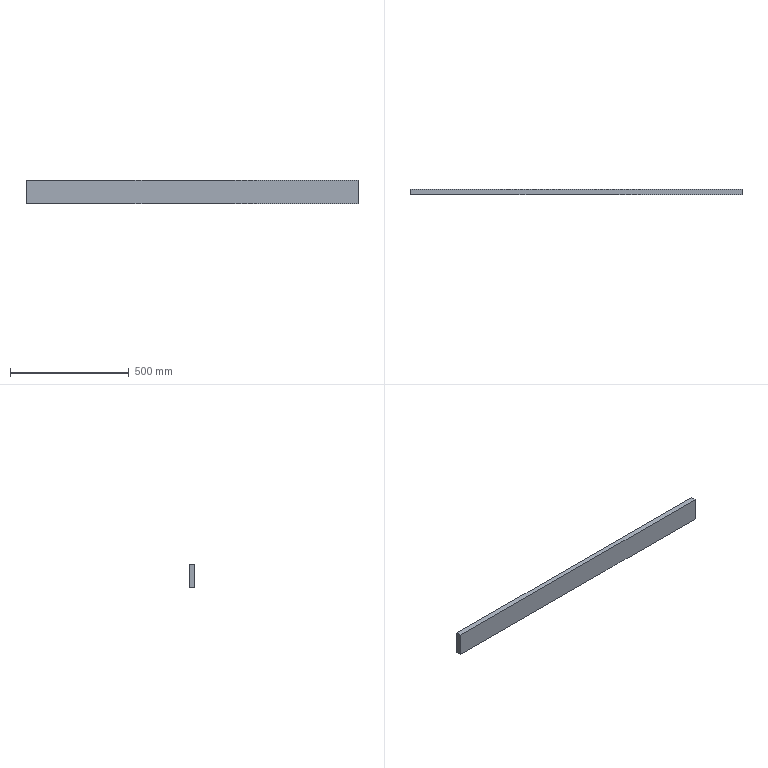Part | SolidWorks | features BaseBody 1 | 1 solid | 6 faces | box 1400 x 22 x 100 mm | volume 3080000 mm3 | plane 6
STEP:
#1=CARTESIAN_POINT('',(700.,132.,317.5));
#2=VERTEX_POINT('',#1);
#3=CARTESIAN_POINT('',(-700.,132.,317.5));
#4=VERTEX_POINT('',#3);
#5=CARTESIAN_POINT('',(0.,132.,317.5));
#6=DIRECTION('',(-1.,0.,0.));
#7=VECTOR('',#6,1000.);
#8=LINE('',#5,#7);
#9=EDGE_CURVE('',#2,#4,#8,.T.);
#10=ORIENTED_EDGE('',*,*,#9,.T.);
#11=CARTESIAN_POINT('',(-700.,132.,417.5));
#12=VERTEX_POINT('',#11);
#13=CARTESIAN_POINT('',(-700.,132.,223.));
#14=DIRECTION('',(0.,0.,1.));
#15=VECTOR('',#14,1000.);
#16=LINE('',#13,#15);
#17=EDGE_CURVE('',#4,#12,#16,.T.);
#18=ORIENTED_EDGE('',*,*,#17,.T.);
#19=CARTESIAN_POINT('',(700.,132.,417.5));
#20=VERTEX_POINT('',#19);
#21=CARTESIAN_POINT('',(0.,132.,417.5));
#22=DIRECTION('',(1.,0.,0.));
#23=VECTOR('',#22,1000.);
#24=LINE('',#21,#23);
#25=EDGE_CURVE('',#12,#20,#24,.T.);
#26=ORIENTED_EDGE('',*,*,#25,.T.);
#27=CARTESIAN_POINT('',(700.,132.,223.));
#28=DIRECTION('',(0.,0.,-1.));
#29=VECTOR('',#28,1000.);
#30=LINE('',#27,#29);
#31=EDGE_CURVE('',#20,#2,#30,.T.);
#32=ORIENTED_EDGE('',*,*,#31,.T.);
#33=EDGE_LOOP('',(#10,#18,#26,#32));
#34=FACE_OUTER_BOUND('',#33,.T.);
#35=CARTESIAN_POINT('',(0.,132.,223.));
#36=DIRECTION('',(0.,1.,0.));
#37=DIRECTION('',(0.,0.,1.));
#38=AXIS2_PLACEMENT_3D('',#35,#36,#37);
#39=PLANE('',#38);
#40=ADVANCED_FACE('',(#34),#39,.T.);
#41=CARTESIAN_POINT('',(-700.,110.,317.5));
#42=VERTEX_POINT('',#41);
#43=CARTESIAN_POINT('',(-700.,102.,317.5));
#44=DIRECTION('',(0.,-1.,0.));
#45=VECTOR('',#44,1000.);
#46=LINE('',#43,#45);
#47=EDGE_CURVE('',#4,#42,#46,.T.);
#48=ORIENTED_EDGE('',*,*,#47,.T.);
#49=CARTESIAN_POINT('',(-700.,110.,417.5));
#50=VERTEX_POINT('',#49);
#51=CARTESIAN_POINT('',(-700.,110.,223.));
#52=DIRECTION('',(0.,0.,1.));
#53=VECTOR('',#52,1000.);
#54=LINE('',#51,#53);
#55=EDGE_CURVE('',#42,#50,#54,.T.);
#56=ORIENTED_EDGE('',*,*,#55,.T.);
#57=CARTESIAN_POINT('',(-700.,102.,417.5));
#58=DIRECTION('',(0.,1.,0.));
#59=VECTOR('',#58,1000.);
#60=LINE('',#57,#59);
#61=EDGE_CURVE('',#50,#12,#60,.T.);
#62=ORIENTED_EDGE('',*,*,#61,.T.);
#63=ORIENTED_EDGE('',*,*,#17,.F.);
#64=EDGE_LOOP('',(#48,#56,#62,#63));
#65=FACE_OUTER_BOUND('',#64,.T.);
#66=CARTESIAN_POINT('',(-700.,102.,223.));
#67=DIRECTION('',(-1.,0.,0.));
#68=DIRECTION('',(0.,0.,1.));
#69=AXIS2_PLACEMENT_3D('',#66,#67,#68);
#70=PLANE('',#69);
#71=ADVANCED_FACE('',(#65),#70,.T.);
#72=ORIENTED_EDGE('',*,*,#9,.F.);
#73=CARTESIAN_POINT('',(700.,110.,317.5));
#74=VERTEX_POINT('',#73);
#75=CARTESIAN_POINT('',(700.,138.5,317.5));
#76=DIRECTION('',(0.,-1.,0.));
#77=VECTOR('',#76,1000.);
#78=LINE('',#75,#77);
#79=EDGE_CURVE('',#2,#74,#78,.T.);
#80=ORIENTED_EDGE('',*,*,#79,.T.);
#81=CARTESIAN_POINT('',(658.479,110.,317.5));
#82=DIRECTION('',(-1.,0.,0.));
#83=VECTOR('',#82,1000.);
#84=LINE('',#81,#83);
#85=EDGE_CURVE('',#74,#42,#84,.T.);
#86=ORIENTED_EDGE('',*,*,#85,.T.);
#87=ORIENTED_EDGE('',*,*,#47,.F.);
#88=EDGE_LOOP('',(#72,#80,#86,#87));
#89=FACE_OUTER_BOUND('',#88,.T.);
#90=CARTESIAN_POINT('',(658.479,138.5,317.5));
#91=DIRECTION('',(0.,0.,-1.));
#92=DIRECTION('',(-1.,0.,0.));
#93=AXIS2_PLACEMENT_3D('',#90,#91,#92);
#94=PLANE('',#93);
#95=ADVANCED_FACE('',(#89),#94,.T.);
#96=CARTESIAN_POINT('',(700.,110.,417.5));
#97=VERTEX_POINT('',#96);
#98=CARTESIAN_POINT('',(700.,110.,223.));
#99=DIRECTION('',(0.,0.,-1.));
#100=VECTOR('',#99,1000.);
#101=LINE('',#98,#100);
#102=EDGE_CURVE('',#97,#74,#101,.T.);
#103=ORIENTED_EDGE('',*,*,#102,.T.);
#104=ORIENTED_EDGE('',*,*,#79,.F.);
#105=ORIENTED_EDGE('',*,*,#31,.F.);
#106=CARTESIAN_POINT('',(700.,102.,417.5));
#107=DIRECTION('',(0.,-1.,0.));
#108=VECTOR('',#107,1000.);
#109=LINE('',#106,#108);
#110=EDGE_CURVE('',#20,#97,#109,.T.);
#111=ORIENTED_EDGE('',*,*,#110,.T.);
#112=EDGE_LOOP('',(#103,#104,#105,#111));
#113=FACE_OUTER_BOUND('',#112,.T.);
#114=CARTESIAN_POINT('',(700.,102.,223.));
#115=DIRECTION('',(1.,0.,0.));
#116=DIRECTION('',(0.,0.,-1.));
#117=AXIS2_PLACEMENT_3D('',#114,#115,#116);
#118=PLANE('',#117);
#119=ADVANCED_FACE('',(#113),#118,.T.);
#120=ORIENTED_EDGE('',*,*,#61,.F.);
#121=CARTESIAN_POINT('',(658.479,110.,417.5));
#122=DIRECTION('',(1.,0.,0.));
#123=VECTOR('',#122,1000.);
#124=LINE('',#121,#123);
#125=EDGE_CURVE('',#50,#97,#124,.T.);
#126=ORIENTED_EDGE('',*,*,#125,.T.);
#127=ORIENTED_EDGE('',*,*,#110,.F.);
#128=ORIENTED_EDGE('',*,*,#25,.F.);
#129=EDGE_LOOP('',(#120,#126,#127,#128));
#130=FACE_OUTER_BOUND('',#129,.T.);
#131=CARTESIAN_POINT('',(658.479,142.5,417.5));
#132=DIRECTION('',(0.,0.,1.));
#133=DIRECTION('',(1.,0.,0.));
#134=AXIS2_PLACEMENT_3D('',#131,#132,#133);
#135=PLANE('',#134);
#136=ADVANCED_FACE('',(#130),#135,.T.);
#137=ORIENTED_EDGE('',*,*,#55,.F.);
#138=ORIENTED_EDGE('',*,*,#85,.F.);
#139=ORIENTED_EDGE('',*,*,#102,.F.);
#140=ORIENTED_EDGE('',*,*,#125,.F.);
#141=EDGE_LOOP('',(#137,#138,#139,#140));
#142=FACE_OUTER_BOUND('',#141,.T.);
#143=CARTESIAN_POINT('',(637.958,110.,407.3));
#144=DIRECTION('',(0.,1.,0.));
#145=DIRECTION('',(0.,0.,1.));
#146=AXIS2_PLACEMENT_3D('',#143,#144,#145);
#147=PLANE('',#146);
#148=ADVANCED_FACE('',(#142),#147,.F.);
#149=CLOSED_SHELL('',(#40,#71,#95,#119,#136,#148));
#150=MANIFOLD_SOLID_BREP('',#149);
#151=CARTESIAN_POINT('',(0.,0.,0.));
#152=DIRECTION('',(0.,0.,1.));
#153=DIRECTION('',(1.,0.,0.));
#154=AXIS2_PLACEMENT_3D('',#151,#152,#153);
#155=(LENGTH_UNIT()NAMED_UNIT(*)SI_UNIT(.MILLI.,.METRE.));
#156=UNCERTAINTY_MEASURE_WITH_UNIT(LENGTH_MEASURE(0.00001),#155,'','');
#157=(NAMED_UNIT(*)PLANE_ANGLE_UNIT()SI_UNIT($,.RADIAN.));
#158=(NAMED_UNIT(*)SI_UNIT($,.STERADIAN.)SOLID_ANGLE_UNIT());
#159=(GEOMETRIC_REPRESENTATION_CONTEXT(3)GLOBAL_UNCERTAINTY_ASSIGNED_CONTEXT((#156))GLOBAL_UNIT_ASSIGNED_CONTEXT((#155,#157,#158))REPRESENTATION_CONTEXT('',''));
#160=ADVANCED_BREP_SHAPE_REPRESENTATION('',(#150,#154),#159);